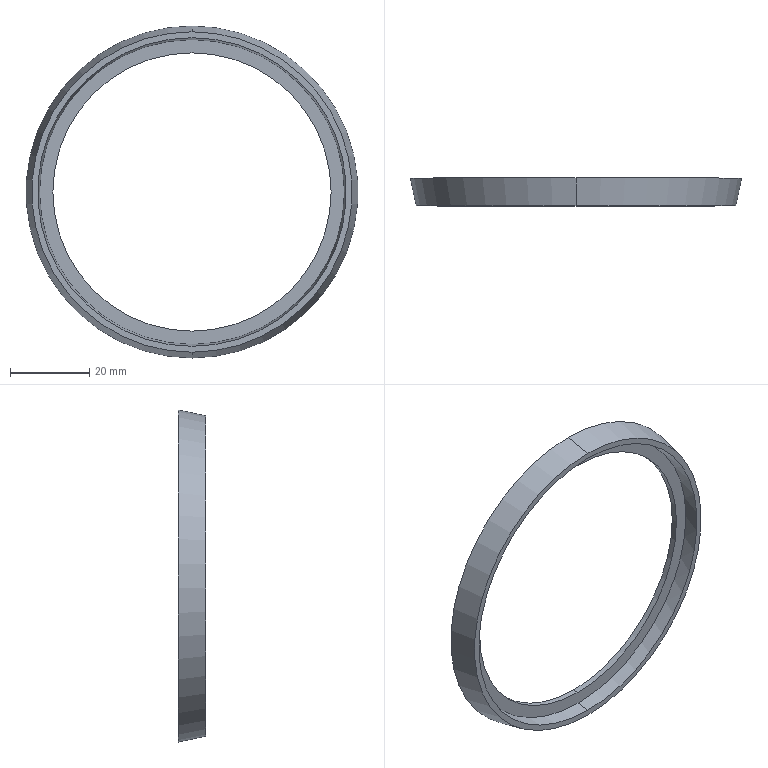Part | NX | features solid 2 | 1 solid | 12 faces | box 83.853 x 7 x 83.853 mm | volume 5165 mm3 | cone 6 | plane 4 | cylinder 2 | commonest cylinder face diameters 70.29 x2
STEP:
#1=CARTESIAN_POINT('',(-190.,-15.379,-890.275));
#2=VERTEX_POINT('',#1);
#3=CARTESIAN_POINT('',(-190.,-13.379,-888.574));
#4=VERTEX_POINT('',#3);
#5=CARTESIAN_POINT('',(-190.,-13.379,-888.574));
#6=DIRECTION('',(0.,-0.7617,-0.648));
#7=VECTOR('',#6,1000.);
#8=LINE('',#5,#7);
#9=EDGE_CURVE('',#2,#4,#8,.F.);
#10=ORIENTED_EDGE('',*,*,#9,.T.);
#11=CARTESIAN_POINT('',(-190.,-13.379,-969.426));
#12=VERTEX_POINT('',#11);
#13=CARTESIAN_POINT('',(-190.,-13.379,-929.));
#14=DIRECTION('',(0.,1.,0.));
#15=DIRECTION('',(0.,0.,1.));
#16=AXIS2_PLACEMENT_3D('',#13,#14,#15);
#17=CIRCLE('',#16,40.426);
#18=EDGE_CURVE('',#4,#12,#17,.T.);
#19=ORIENTED_EDGE('',*,*,#18,.T.);
#20=CARTESIAN_POINT('',(-190.,-15.379,-967.725));
#21=VERTEX_POINT('',#20);
#22=CARTESIAN_POINT('',(-190.,-13.379,-969.426));
#23=DIRECTION('',(0.,-0.7617,0.648));
#24=VECTOR('',#23,1000.);
#25=LINE('',#22,#24);
#26=EDGE_CURVE('',#12,#21,#25,.T.);
#27=ORIENTED_EDGE('',*,*,#26,.T.);
#28=CARTESIAN_POINT('',(-190.,-15.379,-929.));
#29=DIRECTION('',(0.,-1.,0.));
#30=DIRECTION('',(0.,0.,-1.));
#31=AXIS2_PLACEMENT_3D('',#28,#29,#30);
#32=CIRCLE('',#31,38.725);
#33=EDGE_CURVE('',#21,#2,#32,.T.);
#34=ORIENTED_EDGE('',*,*,#33,.T.);
#35=EDGE_LOOP('',(#10,#19,#27,#34));
#36=FACE_BOUND('',#35,.T.);
#37=CARTESIAN_POINT('',(-190.,-14.379,-929.));
#38=DIRECTION('',(0.,1.,0.));
#39=DIRECTION('',(0.,0.,1.));
#40=AXIS2_PLACEMENT_3D('',#37,#38,#39);
#41=CONICAL_SURFACE('',#40,39.576,0.7049);
#42=ADVANCED_FACE('',(#36),#41,.F.);
#43=ORIENTED_EDGE('',*,*,#33,.F.);
#44=CARTESIAN_POINT('',(-190.,-15.379,-929.));
#45=DIRECTION('',(0.,-1.,0.));
#46=DIRECTION('',(0.,0.,1.));
#47=AXIS2_PLACEMENT_3D('',#44,#45,#46);
#48=CIRCLE('',#47,38.725);
#49=EDGE_CURVE('',#2,#21,#48,.T.);
#50=ORIENTED_EDGE('',*,*,#49,.F.);
#51=EDGE_LOOP('',(#43,#50));
#52=FACE_BOUND('',#51,.T.);
#53=CARTESIAN_POINT('',(-190.,-15.379,-964.145));
#54=VERTEX_POINT('',#53);
#55=CARTESIAN_POINT('',(-190.,-15.379,-893.855));
#56=VERTEX_POINT('',#55);
#57=CARTESIAN_POINT('',(-190.,-15.379,-929.));
#58=DIRECTION('',(0.,1.,0.));
#59=DIRECTION('',(0.,0.,-1.));
#60=AXIS2_PLACEMENT_3D('',#57,#58,#59);
#61=CIRCLE('',#60,35.145);
#62=EDGE_CURVE('',#54,#56,#61,.T.);
#63=ORIENTED_EDGE('',*,*,#62,.F.);
#64=CARTESIAN_POINT('',(-190.,-15.379,-929.));
#65=DIRECTION('',(0.,1.,0.));
#66=DIRECTION('',(0.,0.,1.));
#67=AXIS2_PLACEMENT_3D('',#64,#65,#66);
#68=CIRCLE('',#67,35.145);
#69=EDGE_CURVE('',#56,#54,#68,.T.);
#70=ORIENTED_EDGE('',*,*,#69,.F.);
#71=EDGE_LOOP('',(#63,#70));
#72=FACE_BOUND('',#71,.T.);
#73=CARTESIAN_POINT('',(-190.,-15.379,-929.));
#74=DIRECTION('',(0.,-1.,0.));
#75=DIRECTION('',(0.,0.,-1.));
#76=AXIS2_PLACEMENT_3D('',#73,#74,#75);
#77=PLANE('',#76);
#78=ADVANCED_FACE('',(#52,#72),#77,.F.);
#79=ORIENTED_EDGE('',*,*,#49,.T.);
#80=ORIENTED_EDGE('',*,*,#26,.F.);
#81=CARTESIAN_POINT('',(-190.,-13.379,-929.));
#82=DIRECTION('',(0.,1.,0.));
#83=DIRECTION('',(0.,0.,-1.));
#84=AXIS2_PLACEMENT_3D('',#81,#82,#83);
#85=CIRCLE('',#84,40.426);
#86=EDGE_CURVE('',#12,#4,#85,.T.);
#87=ORIENTED_EDGE('',*,*,#86,.T.);
#88=ORIENTED_EDGE('',*,*,#9,.F.);
#89=EDGE_LOOP('',(#79,#80,#87,#88));
#90=FACE_BOUND('',#89,.T.);
#91=CARTESIAN_POINT('',(-190.,-14.379,-929.));
#92=DIRECTION('',(0.,1.,0.));
#93=DIRECTION('',(0.,0.,1.));
#94=AXIS2_PLACEMENT_3D('',#91,#92,#93);
#95=CONICAL_SURFACE('',#94,39.576,0.7049);
#96=ADVANCED_FACE('',(#90),#95,.F.);
#97=CARTESIAN_POINT('',(-190.,-13.379,-887.074));
#98=VERTEX_POINT('',#97);
#99=CARTESIAN_POINT('',(-190.,-13.379,-970.926));
#100=VERTEX_POINT('',#99);
#101=CARTESIAN_POINT('',(-190.,-13.379,-929.));
#102=DIRECTION('',(0.,-1.,0.));
#103=DIRECTION('',(0.,0.,1.));
#104=AXIS2_PLACEMENT_3D('',#101,#102,#103);
#105=CIRCLE('',#104,41.926);
#106=EDGE_CURVE('',#98,#100,#105,.T.);
#107=ORIENTED_EDGE('',*,*,#106,.F.);
#108=CARTESIAN_POINT('',(-190.,-13.379,-929.));
#109=DIRECTION('',(0.,-1.,0.));
#110=DIRECTION('',(0.,0.,-1.));
#111=AXIS2_PLACEMENT_3D('',#108,#109,#110);
#112=CIRCLE('',#111,41.926);
#113=EDGE_CURVE('',#100,#98,#112,.T.);
#114=ORIENTED_EDGE('',*,*,#113,.F.);
#115=EDGE_LOOP('',(#107,#114));
#116=FACE_BOUND('',#115,.T.);
#117=ORIENTED_EDGE('',*,*,#18,.F.);
#118=ORIENTED_EDGE('',*,*,#86,.F.);
#119=EDGE_LOOP('',(#117,#118));
#120=FACE_BOUND('',#119,.T.);
#121=CARTESIAN_POINT('',(-190.,-13.379,-929.));
#122=DIRECTION('',(0.,-1.,0.));
#123=DIRECTION('',(0.,0.,-1.));
#124=AXIS2_PLACEMENT_3D('',#121,#122,#123);
#125=PLANE('',#124);
#126=ADVANCED_FACE('',(#116,#120),#125,.F.);
#127=CARTESIAN_POINT('',(-190.,-20.379,-888.533));
#128=VERTEX_POINT('',#127);
#129=CARTESIAN_POINT('',(-190.,-20.379,-969.467));
#130=VERTEX_POINT('',#129);
#131=CARTESIAN_POINT('',(-190.,-20.379,-929.));
#132=DIRECTION('',(0.,1.,0.));
#133=DIRECTION('',(0.,0.,1.));
#134=AXIS2_PLACEMENT_3D('',#131,#132,#133);
#135=CIRCLE('',#134,40.467);
#136=EDGE_CURVE('',#128,#130,#135,.T.);
#137=ORIENTED_EDGE('',*,*,#136,.T.);
#138=CARTESIAN_POINT('',(-190.,-13.379,-970.926));
#139=DIRECTION('',(0.,-0.9789,0.2042));
#140=VECTOR('',#139,1000.);
#141=LINE('',#138,#140);
#142=EDGE_CURVE('',#130,#100,#141,.F.);
#143=ORIENTED_EDGE('',*,*,#142,.T.);
#144=ORIENTED_EDGE('',*,*,#113,.T.);
#145=CARTESIAN_POINT('',(-190.,-13.379,-887.074));
#146=DIRECTION('',(0.,-0.9789,-0.2042));
#147=VECTOR('',#146,1000.);
#148=LINE('',#145,#147);
#149=EDGE_CURVE('',#98,#128,#148,.T.);
#150=ORIENTED_EDGE('',*,*,#149,.T.);
#151=EDGE_LOOP('',(#137,#143,#144,#150));
#152=FACE_BOUND('',#151,.T.);
#153=CARTESIAN_POINT('',(-190.,-16.879,-929.));
#154=DIRECTION('',(0.,1.,0.));
#155=DIRECTION('',(0.,0.,1.));
#156=AXIS2_PLACEMENT_3D('',#153,#154,#155);
#157=CONICAL_SURFACE('',#156,41.197,0.2056);
#158=ADVANCED_FACE('',(#152),#157,.T.);
#159=ORIENTED_EDGE('',*,*,#149,.F.);
#160=ORIENTED_EDGE('',*,*,#106,.T.);
#161=ORIENTED_EDGE('',*,*,#142,.F.);
#162=CARTESIAN_POINT('',(-190.,-20.379,-929.));
#163=DIRECTION('',(0.,1.,0.));
#164=DIRECTION('',(0.,0.,-1.));
#165=AXIS2_PLACEMENT_3D('',#162,#163,#164);
#166=CIRCLE('',#165,40.467);
#167=EDGE_CURVE('',#130,#128,#166,.T.);
#168=ORIENTED_EDGE('',*,*,#167,.T.);
#169=EDGE_LOOP('',(#159,#160,#161,#168));
#170=FACE_BOUND('',#169,.T.);
#171=CARTESIAN_POINT('',(-190.,-16.879,-929.));
#172=DIRECTION('',(0.,1.,0.));
#173=DIRECTION('',(0.,0.,1.));
#174=AXIS2_PLACEMENT_3D('',#171,#172,#173);
#175=CONICAL_SURFACE('',#174,41.197,0.2056);
#176=ADVANCED_FACE('',(#170),#175,.T.);
#177=ORIENTED_EDGE('',*,*,#136,.F.);
#178=ORIENTED_EDGE('',*,*,#167,.F.);
#179=EDGE_LOOP('',(#177,#178));
#180=FACE_BOUND('',#179,.T.);
#181=CARTESIAN_POINT('',(-190.,-20.379,-890.033));
#182=VERTEX_POINT('',#181);
#183=CARTESIAN_POINT('',(-190.,-20.379,-967.967));
#184=VERTEX_POINT('',#183);
#185=CARTESIAN_POINT('',(-190.,-20.379,-929.));
#186=DIRECTION('',(0.,-1.,0.));
#187=DIRECTION('',(0.,0.,1.));
#188=AXIS2_PLACEMENT_3D('',#185,#186,#187);
#189=CIRCLE('',#188,38.967);
#190=EDGE_CURVE('',#182,#184,#189,.T.);
#191=ORIENTED_EDGE('',*,*,#190,.F.);
#192=CARTESIAN_POINT('',(-190.,-20.379,-929.));
#193=DIRECTION('',(0.,-1.,0.));
#194=DIRECTION('',(0.,0.,-1.));
#195=AXIS2_PLACEMENT_3D('',#192,#193,#194);
#196=CIRCLE('',#195,38.967);
#197=EDGE_CURVE('',#184,#182,#196,.T.);
#198=ORIENTED_EDGE('',*,*,#197,.F.);
#199=EDGE_LOOP('',(#191,#198));
#200=FACE_BOUND('',#199,.T.);
#201=CARTESIAN_POINT('',(-190.,-20.379,-929.));
#202=DIRECTION('',(0.,-1.,0.));
#203=DIRECTION('',(0.,0.,-1.));
#204=AXIS2_PLACEMENT_3D('',#201,#202,#203);
#205=PLANE('',#204);
#206=ADVANCED_FACE('',(#180,#200),#205,.T.);
#207=CARTESIAN_POINT('',(-190.,-16.879,-967.504));
#208=VERTEX_POINT('',#207);
#209=CARTESIAN_POINT('',(-190.,-20.379,-967.967));
#210=DIRECTION('',(0.,0.9914,0.131));
#211=VECTOR('',#210,1000.);
#212=LINE('',#209,#211);
#213=EDGE_CURVE('',#208,#184,#212,.F.);
#214=ORIENTED_EDGE('',*,*,#213,.T.);
#215=ORIENTED_EDGE('',*,*,#197,.T.);
#216=CARTESIAN_POINT('',(-190.,-16.879,-890.496));
#217=VERTEX_POINT('',#216);
#218=CARTESIAN_POINT('',(-190.,-20.379,-890.033));
#219=DIRECTION('',(0.,0.9914,-0.131));
#220=VECTOR('',#219,1000.);
#221=LINE('',#218,#220);
#222=EDGE_CURVE('',#182,#217,#221,.T.);
#223=ORIENTED_EDGE('',*,*,#222,.T.);
#224=CARTESIAN_POINT('',(-190.,-16.879,-929.));
#225=DIRECTION('',(0.,1.,0.));
#226=DIRECTION('',(0.,0.,1.));
#227=AXIS2_PLACEMENT_3D('',#224,#225,#226);
#228=CIRCLE('',#227,38.504);
#229=EDGE_CURVE('',#217,#208,#228,.T.);
#230=ORIENTED_EDGE('',*,*,#229,.T.);
#231=EDGE_LOOP('',(#214,#215,#223,#230));
#232=FACE_BOUND('',#231,.T.);
#233=CARTESIAN_POINT('',(-190.,-18.629,-929.));
#234=DIRECTION('',(0.,-1.,0.));
#235=DIRECTION('',(0.,0.,-1.));
#236=AXIS2_PLACEMENT_3D('',#233,#234,#235);
#237=CONICAL_SURFACE('',#236,38.735,0.1314);
#238=ADVANCED_FACE('',(#232),#237,.F.);
#239=ORIENTED_EDGE('',*,*,#229,.F.);
#240=CARTESIAN_POINT('',(-190.,-16.879,-929.));
#241=DIRECTION('',(0.,1.,0.));
#242=DIRECTION('',(0.,0.,-1.));
#243=AXIS2_PLACEMENT_3D('',#240,#241,#242);
#244=CIRCLE('',#243,38.504);
#245=EDGE_CURVE('',#208,#217,#244,.T.);
#246=ORIENTED_EDGE('',*,*,#245,.F.);
#247=EDGE_LOOP('',(#239,#246));
#248=FACE_BOUND('',#247,.T.);
#249=CARTESIAN_POINT('',(-190.,-16.879,-893.855));
#250=VERTEX_POINT('',#249);
#251=CARTESIAN_POINT('',(-190.,-16.879,-964.145));
#252=VERTEX_POINT('',#251);
#253=CARTESIAN_POINT('',(-190.,-16.879,-929.));
#254=DIRECTION('',(0.,-1.,0.));
#255=DIRECTION('',(0.,0.,1.));
#256=AXIS2_PLACEMENT_3D('',#253,#254,#255);
#257=CIRCLE('',#256,35.145);
#258=EDGE_CURVE('',#250,#252,#257,.T.);
#259=ORIENTED_EDGE('',*,*,#258,.F.);
#260=CARTESIAN_POINT('',(-190.,-16.879,-929.));
#261=DIRECTION('',(0.,-1.,0.));
#262=DIRECTION('',(0.,0.,-1.));
#263=AXIS2_PLACEMENT_3D('',#260,#261,#262);
#264=CIRCLE('',#263,35.145);
#265=EDGE_CURVE('',#252,#250,#264,.T.);
#266=ORIENTED_EDGE('',*,*,#265,.F.);
#267=EDGE_LOOP('',(#259,#266));
#268=FACE_BOUND('',#267,.T.);
#269=CARTESIAN_POINT('',(-190.,-16.879,-929.));
#270=DIRECTION('',(0.,-1.,0.));
#271=DIRECTION('',(0.,0.,-1.));
#272=AXIS2_PLACEMENT_3D('',#269,#270,#271);
#273=PLANE('',#272);
#274=ADVANCED_FACE('',(#248,#268),#273,.T.);
#275=ORIENTED_EDGE('',*,*,#245,.T.);
#276=ORIENTED_EDGE('',*,*,#222,.F.);
#277=ORIENTED_EDGE('',*,*,#190,.T.);
#278=ORIENTED_EDGE('',*,*,#213,.F.);
#279=EDGE_LOOP('',(#275,#276,#277,#278));
#280=FACE_BOUND('',#279,.T.);
#281=CARTESIAN_POINT('',(-190.,-18.629,-929.));
#282=DIRECTION('',(0.,-1.,0.));
#283=DIRECTION('',(0.,0.,-1.));
#284=AXIS2_PLACEMENT_3D('',#281,#282,#283);
#285=CONICAL_SURFACE('',#284,38.735,0.1314);
#286=ADVANCED_FACE('',(#280),#285,.F.);
#287=CARTESIAN_POINT('',(-190.,-16.879,-964.145));
#288=DIRECTION('',(0.,1.,0.));
#289=VECTOR('',#288,1000.);
#290=LINE('',#287,#289);
#291=EDGE_CURVE('',#54,#252,#290,.F.);
#292=ORIENTED_EDGE('',*,*,#291,.T.);
#293=ORIENTED_EDGE('',*,*,#265,.T.);
#294=CARTESIAN_POINT('',(-190.,-16.879,-893.855));
#295=DIRECTION('',(0.,1.,0.));
#296=VECTOR('',#295,1000.);
#297=LINE('',#294,#296);
#298=EDGE_CURVE('',#250,#56,#297,.T.);
#299=ORIENTED_EDGE('',*,*,#298,.T.);
#300=ORIENTED_EDGE('',*,*,#69,.T.);
#301=EDGE_LOOP('',(#292,#293,#299,#300));
#302=FACE_BOUND('',#301,.T.);
#303=CARTESIAN_POINT('',(-190.,-10.531,-929.));
#304=DIRECTION('',(0.,-1.,0.));
#305=DIRECTION('',(0.,0.,-1.));
#306=AXIS2_PLACEMENT_3D('',#303,#304,#305);
#307=CYLINDRICAL_SURFACE('',#306,35.145);
#308=ADVANCED_FACE('',(#302),#307,.F.);
#309=ORIENTED_EDGE('',*,*,#62,.T.);
#310=ORIENTED_EDGE('',*,*,#298,.F.);
#311=ORIENTED_EDGE('',*,*,#258,.T.);
#312=ORIENTED_EDGE('',*,*,#291,.F.);
#313=EDGE_LOOP('',(#309,#310,#311,#312));
#314=FACE_BOUND('',#313,.T.);
#315=CARTESIAN_POINT('',(-190.,-10.531,-929.));
#316=DIRECTION('',(0.,-1.,0.));
#317=DIRECTION('',(0.,0.,-1.));
#318=AXIS2_PLACEMENT_3D('',#315,#316,#317);
#319=CYLINDRICAL_SURFACE('',#318,35.145);
#320=ADVANCED_FACE('',(#314),#319,.F.);
#321=CLOSED_SHELL('',(#42,#78,#96,#126,#158,#176,#206,#238,#274,#286,#308,#320));
#322=MANIFOLD_SOLID_BREP('',#321);
#323=(LENGTH_UNIT()NAMED_UNIT(*)SI_UNIT(.MILLI.,.METRE.));
#324=UNCERTAINTY_MEASURE_WITH_UNIT(LENGTH_MEASURE(0.00001),#323,'','');
#325=(NAMED_UNIT(*)PLANE_ANGLE_UNIT()SI_UNIT($,.RADIAN.));
#326=(NAMED_UNIT(*)SI_UNIT($,.STERADIAN.)SOLID_ANGLE_UNIT());
#327=(GEOMETRIC_REPRESENTATION_CONTEXT(3)GLOBAL_UNCERTAINTY_ASSIGNED_CONTEXT((#324))GLOBAL_UNIT_ASSIGNED_CONTEXT((#323,#325,#326))REPRESENTATION_CONTEXT('',''));
#328=ADVANCED_BREP_SHAPE_REPRESENTATION('',(#322),#327);